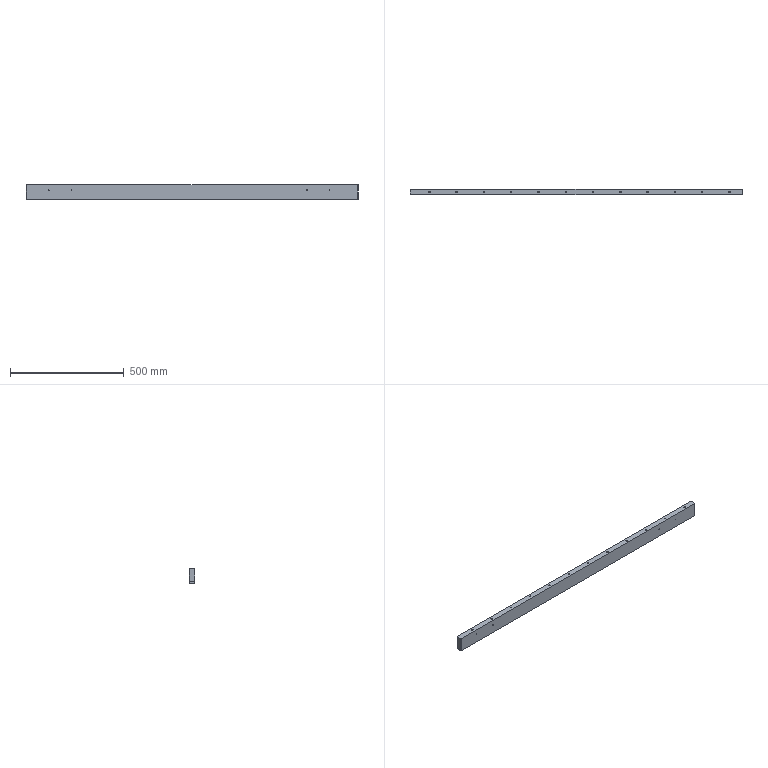Part | NX | 1 solid | 108 faces | box 1460 x 25 x 65 mm | volume 2309213 mm3 | cylinder 57 | cone 29 | plane 22 | commonest cylinder face diameters 4.2 x25 6.6 x12 11 x12 3.3 x8